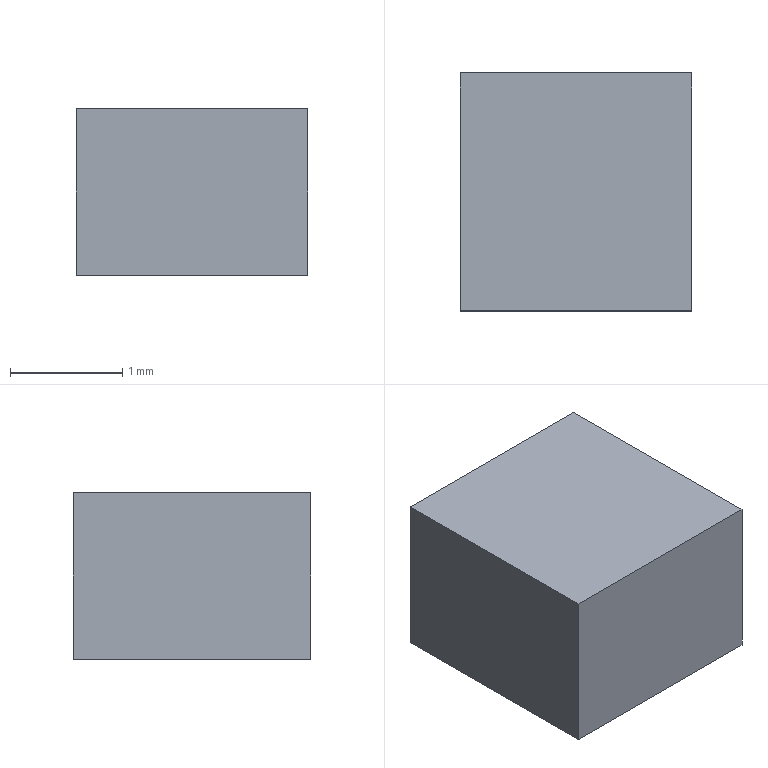Part | Creo | 1 solid | 6 faces | box 2.061 x 2.115 x 1.477 mm | volume 6.439 mm3 | plane 6
STEP:
#1=CARTESIAN_POINT('',(0.,0.,0.));
#2=DIRECTION('',(0.,0.,1.));
#3=DIRECTION('',(1.,0.,0.));
#4=AXIS2_PLACEMENT_3D('',#1,#2,#3);
#5=CARTESIAN_POINT('',(-1.061,-1.005,0.));
#6=VERTEX_POINT('',#5);
#7=CARTESIAN_POINT('',(1.,-1.005,0.));
#8=VERTEX_POINT('',#7);
#9=CARTESIAN_POINT('',(-1.061,-1.005,0.));
#10=DIRECTION('',(1.,0.,0.));
#11=VECTOR('',#10,2.061);
#12=LINE('',#9,#11);
#13=EDGE_CURVE('',#6,#8,#12,.T.);
#14=ORIENTED_EDGE('',*,*,#13,.T.);
#15=CARTESIAN_POINT('',(1.,1.11,0.));
#16=VERTEX_POINT('',#15);
#17=CARTESIAN_POINT('',(1.,-1.005,0.));
#18=DIRECTION('',(0.,1.,0.));
#19=VECTOR('',#18,2.115);
#20=LINE('',#17,#19);
#21=EDGE_CURVE('',#8,#16,#20,.T.);
#22=ORIENTED_EDGE('',*,*,#21,.T.);
#23=CARTESIAN_POINT('',(-1.061,1.11,0.));
#24=VERTEX_POINT('',#23);
#25=CARTESIAN_POINT('',(1.,1.11,0.));
#26=DIRECTION('',(-1.,0.,0.));
#27=VECTOR('',#26,2.061);
#28=LINE('',#25,#27);
#29=EDGE_CURVE('',#16,#24,#28,.T.);
#30=ORIENTED_EDGE('',*,*,#29,.T.);
#31=CARTESIAN_POINT('',(-1.061,1.11,0.));
#32=DIRECTION('',(0.,-1.,0.));
#33=VECTOR('',#32,2.115);
#34=LINE('',#31,#33);
#35=EDGE_CURVE('',#24,#6,#34,.T.);
#36=ORIENTED_EDGE('',*,*,#35,.T.);
#37=EDGE_LOOP('',(#14,#22,#30,#36));
#38=FACE_OUTER_BOUND('',#37,.F.);
#39=CARTESIAN_POINT('',(0.,0.,0.));
#40=DIRECTION('',(0.,0.,1.));
#41=DIRECTION('',(1.,0.,0.));
#42=AXIS2_PLACEMENT_3D('',#39,#40,#41);
#43=PLANE('',#42);
#44=ADVANCED_FACE('',(#38),#43,.F.);
#45=ORIENTED_EDGE('',*,*,#13,.F.);
#46=CARTESIAN_POINT('',(-1.061,-1.005,1.477));
#47=VERTEX_POINT('',#46);
#48=CARTESIAN_POINT('',(-1.061,-1.005,0.));
#49=DIRECTION('',(0.,0.,1.));
#50=VECTOR('',#49,1.477);
#51=LINE('',#48,#50);
#52=EDGE_CURVE('',#6,#47,#51,.T.);
#53=ORIENTED_EDGE('',*,*,#52,.T.);
#54=CARTESIAN_POINT('',(1.,-1.005,1.477));
#55=VERTEX_POINT('',#54);
#56=CARTESIAN_POINT('',(-1.061,-1.005,1.477));
#57=DIRECTION('',(1.,0.,0.));
#58=VECTOR('',#57,2.061);
#59=LINE('',#56,#58);
#60=EDGE_CURVE('',#47,#55,#59,.T.);
#61=ORIENTED_EDGE('',*,*,#60,.T.);
#62=CARTESIAN_POINT('',(1.,-1.005,0.));
#63=DIRECTION('',(0.,0.,1.));
#64=VECTOR('',#63,1.477);
#65=LINE('',#62,#64);
#66=EDGE_CURVE('',#8,#55,#65,.T.);
#67=ORIENTED_EDGE('',*,*,#66,.F.);
#68=EDGE_LOOP('',(#45,#53,#61,#67));
#69=FACE_OUTER_BOUND('',#68,.F.);
#70=CARTESIAN_POINT('',(-1.061,-1.005,0.));
#71=DIRECTION('',(0.,-1.,0.));
#72=DIRECTION('',(1.,0.,0.));
#73=AXIS2_PLACEMENT_3D('',#70,#71,#72);
#74=PLANE('',#73);
#75=ADVANCED_FACE('',(#69),#74,.T.);
#76=ORIENTED_EDGE('',*,*,#35,.F.);
#77=CARTESIAN_POINT('',(-1.061,1.11,1.477));
#78=VERTEX_POINT('',#77);
#79=CARTESIAN_POINT('',(-1.061,1.11,0.));
#80=DIRECTION('',(0.,0.,1.));
#81=VECTOR('',#80,1.477);
#82=LINE('',#79,#81);
#83=EDGE_CURVE('',#24,#78,#82,.T.);
#84=ORIENTED_EDGE('',*,*,#83,.T.);
#85=CARTESIAN_POINT('',(-1.061,1.11,1.477));
#86=DIRECTION('',(0.,-1.,0.));
#87=VECTOR('',#86,2.115);
#88=LINE('',#85,#87);
#89=EDGE_CURVE('',#78,#47,#88,.T.);
#90=ORIENTED_EDGE('',*,*,#89,.T.);
#91=ORIENTED_EDGE('',*,*,#52,.F.);
#92=EDGE_LOOP('',(#76,#84,#90,#91));
#93=FACE_OUTER_BOUND('',#92,.F.);
#94=CARTESIAN_POINT('',(-1.061,1.11,0.));
#95=DIRECTION('',(-1.,0.,0.));
#96=DIRECTION('',(0.,-1.,0.));
#97=AXIS2_PLACEMENT_3D('',#94,#95,#96);
#98=PLANE('',#97);
#99=ADVANCED_FACE('',(#93),#98,.T.);
#100=ORIENTED_EDGE('',*,*,#29,.F.);
#101=CARTESIAN_POINT('',(1.,1.11,1.477));
#102=VERTEX_POINT('',#101);
#103=CARTESIAN_POINT('',(1.,1.11,0.));
#104=DIRECTION('',(0.,0.,1.));
#105=VECTOR('',#104,1.477);
#106=LINE('',#103,#105);
#107=EDGE_CURVE('',#16,#102,#106,.T.);
#108=ORIENTED_EDGE('',*,*,#107,.T.);
#109=CARTESIAN_POINT('',(1.,1.11,1.477));
#110=DIRECTION('',(-1.,0.,0.));
#111=VECTOR('',#110,2.061);
#112=LINE('',#109,#111);
#113=EDGE_CURVE('',#102,#78,#112,.T.);
#114=ORIENTED_EDGE('',*,*,#113,.T.);
#115=ORIENTED_EDGE('',*,*,#83,.F.);
#116=EDGE_LOOP('',(#100,#108,#114,#115));
#117=FACE_OUTER_BOUND('',#116,.F.);
#118=CARTESIAN_POINT('',(1.,1.11,0.));
#119=DIRECTION('',(0.,1.,0.));
#120=DIRECTION('',(-1.,0.,0.));
#121=AXIS2_PLACEMENT_3D('',#118,#119,#120);
#122=PLANE('',#121);
#123=ADVANCED_FACE('',(#117),#122,.T.);
#124=ORIENTED_EDGE('',*,*,#21,.F.);
#125=ORIENTED_EDGE('',*,*,#66,.T.);
#126=CARTESIAN_POINT('',(1.,-1.005,1.477));
#127=DIRECTION('',(0.,1.,0.));
#128=VECTOR('',#127,2.115);
#129=LINE('',#126,#128);
#130=EDGE_CURVE('',#55,#102,#129,.T.);
#131=ORIENTED_EDGE('',*,*,#130,.T.);
#132=ORIENTED_EDGE('',*,*,#107,.F.);
#133=EDGE_LOOP('',(#124,#125,#131,#132));
#134=FACE_OUTER_BOUND('',#133,.F.);
#135=CARTESIAN_POINT('',(1.,-1.005,0.));
#136=DIRECTION('',(1.,0.,0.));
#137=DIRECTION('',(0.,1.,0.));
#138=AXIS2_PLACEMENT_3D('',#135,#136,#137);
#139=PLANE('',#138);
#140=ADVANCED_FACE('',(#134),#139,.T.);
#141=ORIENTED_EDGE('',*,*,#60,.F.);
#142=ORIENTED_EDGE('',*,*,#89,.F.);
#143=ORIENTED_EDGE('',*,*,#113,.F.);
#144=ORIENTED_EDGE('',*,*,#130,.F.);
#145=EDGE_LOOP('',(#141,#142,#143,#144));
#146=FACE_OUTER_BOUND('',#145,.F.);
#147=CARTESIAN_POINT('',(0.,0.,1.477));
#148=DIRECTION('',(0.,0.,1.));
#149=DIRECTION('',(1.,0.,0.));
#150=AXIS2_PLACEMENT_3D('',#147,#148,#149);
#151=PLANE('',#150);
#152=ADVANCED_FACE('',(#146),#151,.T.);
#153=CLOSED_SHELL('',(#44,#75,#99,#123,#140,#152));
#154=MANIFOLD_SOLID_BREP('',#153);
#155=(LENGTH_UNIT()NAMED_UNIT(*)SI_UNIT(.MILLI.,.METRE.));
#156=UNCERTAINTY_MEASURE_WITH_UNIT(LENGTH_MEASURE(0.0003302),#155,'','');
#157=(NAMED_UNIT(*)PLANE_ANGLE_UNIT()SI_UNIT($,.RADIAN.));
#158=PLANE_ANGLE_MEASURE_WITH_UNIT(PLANE_ANGLE_MEASURE(0.01745),#157);
#159=(CONVERSION_BASED_UNIT('DEGREE',#158)NAMED_UNIT(*)PLANE_ANGLE_UNIT());
#160=(NAMED_UNIT(*)SI_UNIT($,.STERADIAN.)SOLID_ANGLE_UNIT());
#161=(GEOMETRIC_REPRESENTATION_CONTEXT(3)GLOBAL_UNCERTAINTY_ASSIGNED_CONTEXT((#156))GLOBAL_UNIT_ASSIGNED_CONTEXT((#155,#159,#160))REPRESENTATION_CONTEXT('',''));
#162=ADVANCED_BREP_SHAPE_REPRESENTATION('',(#4,#154),#161);